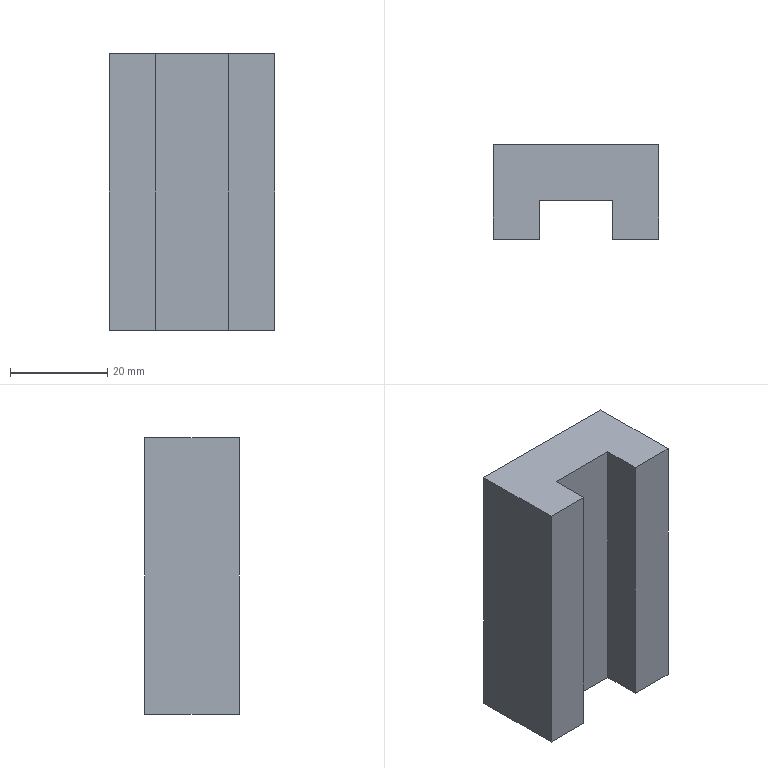Part | SolidWorks | features ICE 2, Extrusion 1 | 1 solid | 22 faces | box 34 x 19.5 x 56.8 mm | volume 30598 mm3 | plane 14 | cylinder 8 | commonest cylinder face diameters 3.6 x8
STEP:
#1=CARTESIAN_POINT('',(-13.,3.75,11.2));
#2=VERTEX_POINT('',#1);
#3=CARTESIAN_POINT('',(-13.,3.75,14.8));
#4=VERTEX_POINT('',#3);
#5=CARTESIAN_POINT('',(-13.,3.75,13.));
#6=DIRECTION('',(0.,1.,0.));
#7=DIRECTION('',(0.,0.,-1.));
#8=AXIS2_PLACEMENT_3D('',#5,#6,#7);
#9=CIRCLE('',#8,1.8);
#10=EDGE_CURVE('',#2,#4,#9,.T.);
#11=ORIENTED_EDGE('',*,*,#10,.F.);
#12=CARTESIAN_POINT('',(-13.,9.75,11.2));
#13=VERTEX_POINT('',#12);
#14=CARTESIAN_POINT('',(-13.,3.75,11.2));
#15=DIRECTION('',(0.,1.,0.));
#16=VECTOR('',#15,1000.);
#17=LINE('',#14,#16);
#18=EDGE_CURVE('',#2,#13,#17,.T.);
#19=ORIENTED_EDGE('',*,*,#18,.T.);
#20=CARTESIAN_POINT('',(-13.,9.75,14.8));
#21=VERTEX_POINT('',#20);
#22=CARTESIAN_POINT('',(-13.,9.75,13.));
#23=DIRECTION('',(0.,1.,0.));
#24=DIRECTION('',(0.,0.,-1.));
#25=AXIS2_PLACEMENT_3D('',#22,#23,#24);
#26=CIRCLE('',#25,1.8);
#27=EDGE_CURVE('',#13,#21,#26,.T.);
#28=ORIENTED_EDGE('',*,*,#27,.T.);
#29=CARTESIAN_POINT('',(-13.,3.75,14.8));
#30=DIRECTION('',(0.,1.,0.));
#31=VECTOR('',#30,1000.);
#32=LINE('',#29,#31);
#33=EDGE_CURVE('',#4,#21,#32,.T.);
#34=ORIENTED_EDGE('',*,*,#33,.F.);
#35=EDGE_LOOP('',(#11,#19,#28,#34));
#36=FACE_OUTER_BOUND('',#35,.T.);
#37=CARTESIAN_POINT('',(-13.,3.75,13.));
#38=DIRECTION('',(0.,1.,0.));
#39=DIRECTION('',(0.,0.,1.));
#40=AXIS2_PLACEMENT_3D('',#37,#38,#39);
#41=CYLINDRICAL_SURFACE('',#40,1.8);
#42=ADVANCED_FACE('',(#36),#41,.F.);
#43=CARTESIAN_POINT('',(13.,3.75,11.2));
#44=VERTEX_POINT('',#43);
#45=CARTESIAN_POINT('',(13.,3.75,14.8));
#46=VERTEX_POINT('',#45);
#47=CARTESIAN_POINT('',(13.,3.75,13.));
#48=DIRECTION('',(0.,1.,0.));
#49=DIRECTION('',(0.,0.,1.));
#50=AXIS2_PLACEMENT_3D('',#47,#48,#49);
#51=CIRCLE('',#50,1.8);
#52=EDGE_CURVE('',#44,#46,#51,.T.);
#53=ORIENTED_EDGE('',*,*,#52,.F.);
#54=CARTESIAN_POINT('',(13.,9.75,11.2));
#55=VERTEX_POINT('',#54);
#56=CARTESIAN_POINT('',(13.,3.75,11.2));
#57=DIRECTION('',(0.,1.,0.));
#58=VECTOR('',#57,1000.);
#59=LINE('',#56,#58);
#60=EDGE_CURVE('',#44,#55,#59,.T.);
#61=ORIENTED_EDGE('',*,*,#60,.T.);
#62=CARTESIAN_POINT('',(13.,9.75,14.8));
#63=VERTEX_POINT('',#62);
#64=CARTESIAN_POINT('',(13.,9.75,13.));
#65=DIRECTION('',(0.,1.,0.));
#66=DIRECTION('',(0.,0.,1.));
#67=AXIS2_PLACEMENT_3D('',#64,#65,#66);
#68=CIRCLE('',#67,1.8);
#69=EDGE_CURVE('',#55,#63,#68,.T.);
#70=ORIENTED_EDGE('',*,*,#69,.T.);
#71=CARTESIAN_POINT('',(13.,3.75,14.8));
#72=DIRECTION('',(0.,1.,0.));
#73=VECTOR('',#72,1000.);
#74=LINE('',#71,#73);
#75=EDGE_CURVE('',#46,#63,#74,.T.);
#76=ORIENTED_EDGE('',*,*,#75,.F.);
#77=EDGE_LOOP('',(#53,#61,#70,#76));
#78=FACE_OUTER_BOUND('',#77,.T.);
#79=CARTESIAN_POINT('',(13.,3.75,13.));
#80=DIRECTION('',(0.,1.,0.));
#81=DIRECTION('',(0.,0.,1.));
#82=AXIS2_PLACEMENT_3D('',#79,#80,#81);
#83=CYLINDRICAL_SURFACE('',#82,1.8);
#84=ADVANCED_FACE('',(#78),#83,.F.);
#85=CARTESIAN_POINT('',(13.,3.75,-14.8));
#86=VERTEX_POINT('',#85);
#87=CARTESIAN_POINT('',(13.,3.75,-11.2));
#88=VERTEX_POINT('',#87);
#89=CARTESIAN_POINT('',(13.,3.75,-13.));
#90=DIRECTION('',(0.,1.,0.));
#91=DIRECTION('',(0.,0.,-1.));
#92=AXIS2_PLACEMENT_3D('',#89,#90,#91);
#93=CIRCLE('',#92,1.8);
#94=EDGE_CURVE('',#86,#88,#93,.T.);
#95=ORIENTED_EDGE('',*,*,#94,.F.);
#96=CARTESIAN_POINT('',(13.,9.75,-14.8));
#97=VERTEX_POINT('',#96);
#98=CARTESIAN_POINT('',(13.,3.75,-14.8));
#99=DIRECTION('',(0.,1.,0.));
#100=VECTOR('',#99,1000.);
#101=LINE('',#98,#100);
#102=EDGE_CURVE('',#86,#97,#101,.T.);
#103=ORIENTED_EDGE('',*,*,#102,.T.);
#104=CARTESIAN_POINT('',(13.,9.75,-11.2));
#105=VERTEX_POINT('',#104);
#106=CARTESIAN_POINT('',(13.,9.75,-13.));
#107=DIRECTION('',(0.,1.,0.));
#108=DIRECTION('',(0.,0.,-1.));
#109=AXIS2_PLACEMENT_3D('',#106,#107,#108);
#110=CIRCLE('',#109,1.8);
#111=EDGE_CURVE('',#97,#105,#110,.T.);
#112=ORIENTED_EDGE('',*,*,#111,.T.);
#113=CARTESIAN_POINT('',(13.,3.75,-11.2));
#114=DIRECTION('',(0.,1.,0.));
#115=VECTOR('',#114,1000.);
#116=LINE('',#113,#115);
#117=EDGE_CURVE('',#88,#105,#116,.T.);
#118=ORIENTED_EDGE('',*,*,#117,.F.);
#119=EDGE_LOOP('',(#95,#103,#112,#118));
#120=FACE_OUTER_BOUND('',#119,.T.);
#121=CARTESIAN_POINT('',(13.,3.75,-13.));
#122=DIRECTION('',(0.,1.,0.));
#123=DIRECTION('',(0.,0.,1.));
#124=AXIS2_PLACEMENT_3D('',#121,#122,#123);
#125=CYLINDRICAL_SURFACE('',#124,1.8);
#126=ADVANCED_FACE('',(#120),#125,.F.);
#127=CARTESIAN_POINT('',(-13.,3.75,-14.8));
#128=VERTEX_POINT('',#127);
#129=CARTESIAN_POINT('',(-13.,3.75,-11.2));
#130=VERTEX_POINT('',#129);
#131=CARTESIAN_POINT('',(-13.,3.75,-13.));
#132=DIRECTION('',(0.,1.,0.));
#133=DIRECTION('',(0.,0.,1.));
#134=AXIS2_PLACEMENT_3D('',#131,#132,#133);
#135=CIRCLE('',#134,1.8);
#136=EDGE_CURVE('',#128,#130,#135,.T.);
#137=ORIENTED_EDGE('',*,*,#136,.F.);
#138=CARTESIAN_POINT('',(-13.,9.75,-14.8));
#139=VERTEX_POINT('',#138);
#140=CARTESIAN_POINT('',(-13.,3.75,-14.8));
#141=DIRECTION('',(0.,1.,0.));
#142=VECTOR('',#141,1000.);
#143=LINE('',#140,#142);
#144=EDGE_CURVE('',#128,#139,#143,.T.);
#145=ORIENTED_EDGE('',*,*,#144,.T.);
#146=CARTESIAN_POINT('',(-13.,9.75,-11.2));
#147=VERTEX_POINT('',#146);
#148=CARTESIAN_POINT('',(-13.,9.75,-13.));
#149=DIRECTION('',(0.,1.,0.));
#150=DIRECTION('',(0.,0.,1.));
#151=AXIS2_PLACEMENT_3D('',#148,#149,#150);
#152=CIRCLE('',#151,1.8);
#153=EDGE_CURVE('',#139,#147,#152,.T.);
#154=ORIENTED_EDGE('',*,*,#153,.T.);
#155=CARTESIAN_POINT('',(-13.,3.75,-11.2));
#156=DIRECTION('',(0.,1.,0.));
#157=VECTOR('',#156,1000.);
#158=LINE('',#155,#157);
#159=EDGE_CURVE('',#130,#147,#158,.T.);
#160=ORIENTED_EDGE('',*,*,#159,.F.);
#161=EDGE_LOOP('',(#137,#145,#154,#160));
#162=FACE_OUTER_BOUND('',#161,.T.);
#163=CARTESIAN_POINT('',(-13.,3.75,-13.));
#164=DIRECTION('',(0.,1.,0.));
#165=DIRECTION('',(0.,0.,1.));
#166=AXIS2_PLACEMENT_3D('',#163,#164,#165);
#167=CYLINDRICAL_SURFACE('',#166,1.8);
#168=ADVANCED_FACE('',(#162),#167,.F.);
#169=CARTESIAN_POINT('',(7.5,-9.75,28.4));
#170=VERTEX_POINT('',#169);
#171=CARTESIAN_POINT('',(17.,-9.75,28.4));
#172=VERTEX_POINT('',#171);
#173=CARTESIAN_POINT('',(-17.,-9.75,28.4));
#174=DIRECTION('',(1.,0.,0.));
#175=VECTOR('',#174,1000.);
#176=LINE('',#173,#175);
#177=EDGE_CURVE('',#170,#172,#176,.T.);
#178=ORIENTED_EDGE('',*,*,#177,.F.);
#179=CARTESIAN_POINT('',(7.5,-9.75,-28.4));
#180=VERTEX_POINT('',#179);
#181=CARTESIAN_POINT('',(7.5,-9.75,-28.4));
#182=DIRECTION('',(0.,0.,1.));
#183=VECTOR('',#182,1000.);
#184=LINE('',#181,#183);
#185=EDGE_CURVE('',#180,#170,#184,.T.);
#186=ORIENTED_EDGE('',*,*,#185,.F.);
#187=CARTESIAN_POINT('',(17.,-9.75,-28.4));
#188=VERTEX_POINT('',#187);
#189=CARTESIAN_POINT('',(-17.,-9.75,-28.4));
#190=DIRECTION('',(1.,0.,0.));
#191=VECTOR('',#190,1000.);
#192=LINE('',#189,#191);
#193=EDGE_CURVE('',#180,#188,#192,.T.);
#194=ORIENTED_EDGE('',*,*,#193,.T.);
#195=CARTESIAN_POINT('',(17.,-9.75,28.4));
#196=DIRECTION('',(0.,0.,-1.));
#197=VECTOR('',#196,1000.);
#198=LINE('',#195,#197);
#199=EDGE_CURVE('',#172,#188,#198,.T.);
#200=ORIENTED_EDGE('',*,*,#199,.F.);
#201=EDGE_LOOP('',(#178,#186,#194,#200));
#202=FACE_OUTER_BOUND('',#201,.T.);
#203=CARTESIAN_POINT('',(-17.,-9.75,28.4));
#204=DIRECTION('',(0.,1.,0.));
#205=DIRECTION('',(0.,0.,1.));
#206=AXIS2_PLACEMENT_3D('',#203,#204,#205);
#207=PLANE('',#206);
#208=ADVANCED_FACE('',(#202),#207,.F.);
#209=CARTESIAN_POINT('',(17.,9.75,-28.4));
#210=VERTEX_POINT('',#209);
#211=CARTESIAN_POINT('',(17.,9.75,-28.4));
#212=DIRECTION('',(0.,1.,0.));
#213=VECTOR('',#212,1000.);
#214=LINE('',#211,#213);
#215=EDGE_CURVE('',#188,#210,#214,.T.);
#216=ORIENTED_EDGE('',*,*,#215,.T.);
#217=CARTESIAN_POINT('',(17.,9.75,28.4));
#218=VERTEX_POINT('',#217);
#219=CARTESIAN_POINT('',(17.,9.75,28.4));
#220=DIRECTION('',(0.,0.,-1.));
#221=VECTOR('',#220,1000.);
#222=LINE('',#219,#221);
#223=EDGE_CURVE('',#218,#210,#222,.T.);
#224=ORIENTED_EDGE('',*,*,#223,.F.);
#225=CARTESIAN_POINT('',(17.,9.75,28.4));
#226=DIRECTION('',(0.,1.,0.));
#227=VECTOR('',#226,1000.);
#228=LINE('',#225,#227);
#229=EDGE_CURVE('',#172,#218,#228,.T.);
#230=ORIENTED_EDGE('',*,*,#229,.F.);
#231=ORIENTED_EDGE('',*,*,#199,.T.);
#232=EDGE_LOOP('',(#216,#224,#230,#231));
#233=FACE_OUTER_BOUND('',#232,.T.);
#234=CARTESIAN_POINT('',(17.,9.75,28.4));
#235=DIRECTION('',(-1.,0.,0.));
#236=DIRECTION('',(0.,-1.,0.));
#237=AXIS2_PLACEMENT_3D('',#234,#235,#236);
#238=PLANE('',#237);
#239=ADVANCED_FACE('',(#233),#238,.F.);
#240=CARTESIAN_POINT('',(-13.,9.75,13.));
#241=DIRECTION('',(0.,1.,0.));
#242=DIRECTION('',(0.,0.,-1.));
#243=AXIS2_PLACEMENT_3D('',#240,#241,#242);
#244=CIRCLE('',#243,1.8);
#245=EDGE_CURVE('',#21,#13,#244,.T.);
#246=ORIENTED_EDGE('',*,*,#245,.F.);
#247=ORIENTED_EDGE('',*,*,#27,.F.);
#248=EDGE_LOOP('',(#246,#247));
#249=FACE_BOUND('',#248,.T.);
#250=CARTESIAN_POINT('',(13.,9.75,13.));
#251=DIRECTION('',(0.,1.,0.));
#252=DIRECTION('',(0.,0.,1.));
#253=AXIS2_PLACEMENT_3D('',#250,#251,#252);
#254=CIRCLE('',#253,1.8);
#255=EDGE_CURVE('',#63,#55,#254,.T.);
#256=ORIENTED_EDGE('',*,*,#255,.F.);
#257=ORIENTED_EDGE('',*,*,#69,.F.);
#258=EDGE_LOOP('',(#256,#257));
#259=FACE_BOUND('',#258,.T.);
#260=CARTESIAN_POINT('',(13.,9.75,-13.));
#261=DIRECTION('',(0.,1.,0.));
#262=DIRECTION('',(0.,0.,-1.));
#263=AXIS2_PLACEMENT_3D('',#260,#261,#262);
#264=CIRCLE('',#263,1.8);
#265=EDGE_CURVE('',#105,#97,#264,.T.);
#266=ORIENTED_EDGE('',*,*,#265,.F.);
#267=ORIENTED_EDGE('',*,*,#111,.F.);
#268=EDGE_LOOP('',(#266,#267));
#269=FACE_BOUND('',#268,.T.);
#270=CARTESIAN_POINT('',(-13.,9.75,-13.));
#271=DIRECTION('',(0.,1.,0.));
#272=DIRECTION('',(0.,0.,1.));
#273=AXIS2_PLACEMENT_3D('',#270,#271,#272);
#274=CIRCLE('',#273,1.8);
#275=EDGE_CURVE('',#147,#139,#274,.T.);
#276=ORIENTED_EDGE('',*,*,#275,.F.);
#277=ORIENTED_EDGE('',*,*,#153,.F.);
#278=EDGE_LOOP('',(#276,#277));
#279=FACE_BOUND('',#278,.T.);
#280=CARTESIAN_POINT('',(-17.,9.75,-28.4));
#281=VERTEX_POINT('',#280);
#282=CARTESIAN_POINT('',(-17.,9.75,-28.4));
#283=DIRECTION('',(-1.,0.,0.));
#284=VECTOR('',#283,1000.);
#285=LINE('',#282,#284);
#286=EDGE_CURVE('',#210,#281,#285,.T.);
#287=ORIENTED_EDGE('',*,*,#286,.T.);
#288=CARTESIAN_POINT('',(-17.,9.75,28.4));
#289=VERTEX_POINT('',#288);
#290=CARTESIAN_POINT('',(-17.,9.75,28.4));
#291=DIRECTION('',(0.,0.,-1.));
#292=VECTOR('',#291,1000.);
#293=LINE('',#290,#292);
#294=EDGE_CURVE('',#289,#281,#293,.T.);
#295=ORIENTED_EDGE('',*,*,#294,.F.);
#296=CARTESIAN_POINT('',(-17.,9.75,28.4));
#297=DIRECTION('',(-1.,0.,0.));
#298=VECTOR('',#297,1000.);
#299=LINE('',#296,#298);
#300=EDGE_CURVE('',#218,#289,#299,.T.);
#301=ORIENTED_EDGE('',*,*,#300,.F.);
#302=ORIENTED_EDGE('',*,*,#223,.T.);
#303=EDGE_LOOP('',(#287,#295,#301,#302));
#304=FACE_OUTER_BOUND('',#303,.T.);
#305=CARTESIAN_POINT('',(-17.,9.75,28.4));
#306=DIRECTION('',(0.,-1.,0.));
#307=DIRECTION('',(0.,0.,-1.));
#308=AXIS2_PLACEMENT_3D('',#305,#306,#307);
#309=PLANE('',#308);
#310=ADVANCED_FACE('',(#249,#259,#269,#279,#304),#309,.F.);
#311=CARTESIAN_POINT('',(-17.,-9.75,-28.4));
#312=VERTEX_POINT('',#311);
#313=CARTESIAN_POINT('',(-17.,9.75,-28.4));
#314=DIRECTION('',(0.,-1.,0.));
#315=VECTOR('',#314,1000.);
#316=LINE('',#313,#315);
#317=EDGE_CURVE('',#281,#312,#316,.T.);
#318=ORIENTED_EDGE('',*,*,#317,.T.);
#319=CARTESIAN_POINT('',(-17.,-9.75,28.4));
#320=VERTEX_POINT('',#319);
#321=CARTESIAN_POINT('',(-17.,-9.75,28.4));
#322=DIRECTION('',(0.,0.,-1.));
#323=VECTOR('',#322,1000.);
#324=LINE('',#321,#323);
#325=EDGE_CURVE('',#320,#312,#324,.T.);
#326=ORIENTED_EDGE('',*,*,#325,.F.);
#327=CARTESIAN_POINT('',(-17.,9.75,28.4));
#328=DIRECTION('',(0.,-1.,0.));
#329=VECTOR('',#328,1000.);
#330=LINE('',#327,#329);
#331=EDGE_CURVE('',#289,#320,#330,.T.);
#332=ORIENTED_EDGE('',*,*,#331,.F.);
#333=ORIENTED_EDGE('',*,*,#294,.T.);
#334=EDGE_LOOP('',(#318,#326,#332,#333));
#335=FACE_OUTER_BOUND('',#334,.T.);
#336=CARTESIAN_POINT('',(-17.,9.75,28.4));
#337=DIRECTION('',(1.,0.,0.));
#338=DIRECTION('',(0.,1.,0.));
#339=AXIS2_PLACEMENT_3D('',#336,#337,#338);
#340=PLANE('',#339);
#341=ADVANCED_FACE('',(#335),#340,.F.);
#342=CARTESIAN_POINT('',(-7.5,-9.75,-28.4));
#343=VERTEX_POINT('',#342);
#344=CARTESIAN_POINT('',(-17.,-9.75,-28.4));
#345=DIRECTION('',(1.,0.,0.));
#346=VECTOR('',#345,1000.);
#347=LINE('',#344,#346);
#348=EDGE_CURVE('',#312,#343,#347,.T.);
#349=ORIENTED_EDGE('',*,*,#348,.T.);
#350=CARTESIAN_POINT('',(-7.5,-9.75,28.4));
#351=VERTEX_POINT('',#350);
#352=CARTESIAN_POINT('',(-7.5,-9.75,-28.4));
#353=DIRECTION('',(0.,0.,1.));
#354=VECTOR('',#353,1000.);
#355=LINE('',#352,#354);
#356=EDGE_CURVE('',#343,#351,#355,.T.);
#357=ORIENTED_EDGE('',*,*,#356,.T.);
#358=CARTESIAN_POINT('',(-17.,-9.75,28.4));
#359=DIRECTION('',(1.,0.,0.));
#360=VECTOR('',#359,1000.);
#361=LINE('',#358,#360);
#362=EDGE_CURVE('',#320,#351,#361,.T.);
#363=ORIENTED_EDGE('',*,*,#362,.F.);
#364=ORIENTED_EDGE('',*,*,#325,.T.);
#365=EDGE_LOOP('',(#349,#357,#363,#364));
#366=FACE_OUTER_BOUND('',#365,.T.);
#367=CARTESIAN_POINT('',(-17.,-9.75,28.4));
#368=DIRECTION('',(0.,1.,0.));
#369=DIRECTION('',(0.,0.,1.));
#370=AXIS2_PLACEMENT_3D('',#367,#368,#369);
#371=PLANE('',#370);
#372=ADVANCED_FACE('',(#366),#371,.F.);
#373=CARTESIAN_POINT('',(7.5,-1.75,28.4));
#374=VERTEX_POINT('',#373);
#375=CARTESIAN_POINT('',(7.5,-1.75,28.4));
#376=DIRECTION('',(0.,1.,0.));
#377=VECTOR('',#376,1000.);
#378=LINE('',#375,#377);
#379=EDGE_CURVE('',#170,#374,#378,.T.);
#380=ORIENTED_EDGE('',*,*,#379,.F.);
#381=ORIENTED_EDGE('',*,*,#177,.T.);
#382=ORIENTED_EDGE('',*,*,#229,.T.);
#383=ORIENTED_EDGE('',*,*,#300,.T.);
#384=ORIENTED_EDGE('',*,*,#331,.T.);
#385=ORIENTED_EDGE('',*,*,#362,.T.);
#386=CARTESIAN_POINT('',(-7.5,-1.75,28.4));
#387=VERTEX_POINT('',#386);
#388=CARTESIAN_POINT('',(-7.5,-1.75,28.4));
#389=DIRECTION('',(0.,-1.,0.));
#390=VECTOR('',#389,1000.);
#391=LINE('',#388,#390);
#392=EDGE_CURVE('',#387,#351,#391,.T.);
#393=ORIENTED_EDGE('',*,*,#392,.F.);
#394=CARTESIAN_POINT('',(-7.5,-1.75,28.4));
#395=DIRECTION('',(-1.,0.,0.));
#396=VECTOR('',#395,1000.);
#397=LINE('',#394,#396);
#398=EDGE_CURVE('',#374,#387,#397,.T.);
#399=ORIENTED_EDGE('',*,*,#398,.F.);
#400=EDGE_LOOP('',(#380,#381,#382,#383,#384,#385,#393,#399));
#401=FACE_OUTER_BOUND('',#400,.T.);
#402=CARTESIAN_POINT('',(0.,0.,28.4));
#403=DIRECTION('',(0.,0.,1.));
#404=DIRECTION('',(1.,0.,0.));
#405=AXIS2_PLACEMENT_3D('',#402,#403,#404);
#406=PLANE('',#405);
#407=ADVANCED_FACE('',(#401),#406,.T.);
#408=ORIENTED_EDGE('',*,*,#193,.F.);
#409=CARTESIAN_POINT('',(7.5,-1.75,-28.4));
#410=VERTEX_POINT('',#409);
#411=CARTESIAN_POINT('',(7.5,-1.75,-28.4));
#412=DIRECTION('',(0.,1.,0.));
#413=VECTOR('',#412,1000.);
#414=LINE('',#411,#413);
#415=EDGE_CURVE('',#180,#410,#414,.T.);
#416=ORIENTED_EDGE('',*,*,#415,.T.);
#417=CARTESIAN_POINT('',(-7.5,-1.75,-28.4));
#418=VERTEX_POINT('',#417);
#419=CARTESIAN_POINT('',(-7.5,-1.75,-28.4));
#420=DIRECTION('',(-1.,0.,0.));
#421=VECTOR('',#420,1000.);
#422=LINE('',#419,#421);
#423=EDGE_CURVE('',#410,#418,#422,.T.);
#424=ORIENTED_EDGE('',*,*,#423,.T.);
#425=CARTESIAN_POINT('',(-7.5,-1.75,-28.4));
#426=DIRECTION('',(0.,-1.,0.));
#427=VECTOR('',#426,1000.);
#428=LINE('',#425,#427);
#429=EDGE_CURVE('',#418,#343,#428,.T.);
#430=ORIENTED_EDGE('',*,*,#429,.T.);
#431=ORIENTED_EDGE('',*,*,#348,.F.);
#432=ORIENTED_EDGE('',*,*,#317,.F.);
#433=ORIENTED_EDGE('',*,*,#286,.F.);
#434=ORIENTED_EDGE('',*,*,#215,.F.);
#435=EDGE_LOOP('',(#408,#416,#424,#430,#431,#432,#433,#434));
#436=FACE_OUTER_BOUND('',#435,.T.);
#437=CARTESIAN_POINT('',(0.,0.,-28.4));
#438=DIRECTION('',(0.,0.,1.));
#439=DIRECTION('',(1.,0.,0.));
#440=AXIS2_PLACEMENT_3D('',#437,#438,#439);
#441=PLANE('',#440);
#442=ADVANCED_FACE('',(#436),#441,.F.);
#443=CARTESIAN_POINT('',(7.5,-1.75,-28.4));
#444=DIRECTION('',(0.,0.,1.));
#445=VECTOR('',#444,1000.);
#446=LINE('',#443,#445);
#447=EDGE_CURVE('',#410,#374,#446,.T.);
#448=ORIENTED_EDGE('',*,*,#447,.F.);
#449=ORIENTED_EDGE('',*,*,#415,.F.);
#450=ORIENTED_EDGE('',*,*,#185,.T.);
#451=ORIENTED_EDGE('',*,*,#379,.T.);
#452=EDGE_LOOP('',(#448,#449,#450,#451));
#453=FACE_OUTER_BOUND('',#452,.T.);
#454=CARTESIAN_POINT('',(7.5,-1.75,-28.4));
#455=DIRECTION('',(1.,0.,0.));
#456=DIRECTION('',(0.,1.,0.));
#457=AXIS2_PLACEMENT_3D('',#454,#455,#456);
#458=PLANE('',#457);
#459=ADVANCED_FACE('',(#453),#458,.F.);
#460=ORIENTED_EDGE('',*,*,#356,.F.);
#461=ORIENTED_EDGE('',*,*,#429,.F.);
#462=CARTESIAN_POINT('',(-7.5,-1.75,-28.4));
#463=DIRECTION('',(0.,0.,1.));
#464=VECTOR('',#463,1000.);
#465=LINE('',#462,#464);
#466=EDGE_CURVE('',#418,#387,#465,.T.);
#467=ORIENTED_EDGE('',*,*,#466,.T.);
#468=ORIENTED_EDGE('',*,*,#392,.T.);
#469=EDGE_LOOP('',(#460,#461,#467,#468));
#470=FACE_OUTER_BOUND('',#469,.T.);
#471=CARTESIAN_POINT('',(-7.5,-1.75,-28.4));
#472=DIRECTION('',(-1.,0.,0.));
#473=DIRECTION('',(0.,-1.,0.));
#474=AXIS2_PLACEMENT_3D('',#471,#472,#473);
#475=PLANE('',#474);
#476=ADVANCED_FACE('',(#470),#475,.F.);
#477=ORIENTED_EDGE('',*,*,#466,.F.);
#478=ORIENTED_EDGE('',*,*,#423,.F.);
#479=ORIENTED_EDGE('',*,*,#447,.T.);
#480=ORIENTED_EDGE('',*,*,#398,.T.);
#481=EDGE_LOOP('',(#477,#478,#479,#480));
#482=FACE_OUTER_BOUND('',#481,.T.);
#483=CARTESIAN_POINT('',(-7.5,-1.75,-28.4));
#484=DIRECTION('',(0.,1.,0.));
#485=DIRECTION('',(0.,0.,1.));
#486=AXIS2_PLACEMENT_3D('',#483,#484,#485);
#487=PLANE('',#486);
#488=ADVANCED_FACE('',(#482),#487,.F.);
#489=ORIENTED_EDGE('',*,*,#144,.F.);
#490=CARTESIAN_POINT('',(-13.,3.75,-13.));
#491=DIRECTION('',(0.,1.,0.));
#492=DIRECTION('',(0.,0.,1.));
#493=AXIS2_PLACEMENT_3D('',#490,#491,#492);
#494=CIRCLE('',#493,1.8);
#495=EDGE_CURVE('',#130,#128,#494,.T.);
#496=ORIENTED_EDGE('',*,*,#495,.F.);
#497=ORIENTED_EDGE('',*,*,#159,.T.);
#498=ORIENTED_EDGE('',*,*,#275,.T.);
#499=EDGE_LOOP('',(#489,#496,#497,#498));
#500=FACE_OUTER_BOUND('',#499,.T.);
#501=CARTESIAN_POINT('',(-13.,3.75,-13.));
#502=DIRECTION('',(0.,1.,0.));
#503=DIRECTION('',(0.,0.,1.));
#504=AXIS2_PLACEMENT_3D('',#501,#502,#503);
#505=CYLINDRICAL_SURFACE('',#504,1.8);
#506=ADVANCED_FACE('',(#500),#505,.F.);
#507=ORIENTED_EDGE('',*,*,#495,.T.);
#508=ORIENTED_EDGE('',*,*,#136,.T.);
#509=EDGE_LOOP('',(#507,#508));
#510=FACE_OUTER_BOUND('',#509,.T.);
#511=CARTESIAN_POINT('',(-13.,3.75,-13.));
#512=DIRECTION('',(0.,1.,0.));
#513=DIRECTION('',(0.,0.,1.));
#514=AXIS2_PLACEMENT_3D('',#511,#512,#513);
#515=PLANE('',#514);
#516=ADVANCED_FACE('',(#510),#515,.T.);
#517=ORIENTED_EDGE('',*,*,#102,.F.);
#518=CARTESIAN_POINT('',(13.,3.75,-13.));
#519=DIRECTION('',(0.,1.,0.));
#520=DIRECTION('',(0.,0.,-1.));
#521=AXIS2_PLACEMENT_3D('',#518,#519,#520);
#522=CIRCLE('',#521,1.8);
#523=EDGE_CURVE('',#88,#86,#522,.T.);
#524=ORIENTED_EDGE('',*,*,#523,.F.);
#525=ORIENTED_EDGE('',*,*,#117,.T.);
#526=ORIENTED_EDGE('',*,*,#265,.T.);
#527=EDGE_LOOP('',(#517,#524,#525,#526));
#528=FACE_OUTER_BOUND('',#527,.T.);
#529=CARTESIAN_POINT('',(13.,3.75,-13.));
#530=DIRECTION('',(0.,1.,0.));
#531=DIRECTION('',(0.,0.,1.));
#532=AXIS2_PLACEMENT_3D('',#529,#530,#531);
#533=CYLINDRICAL_SURFACE('',#532,1.8);
#534=ADVANCED_FACE('',(#528),#533,.F.);
#535=ORIENTED_EDGE('',*,*,#523,.T.);
#536=ORIENTED_EDGE('',*,*,#94,.T.);
#537=EDGE_LOOP('',(#535,#536));
#538=FACE_OUTER_BOUND('',#537,.T.);
#539=CARTESIAN_POINT('',(13.,3.75,-13.));
#540=DIRECTION('',(0.,-1.,0.));
#541=DIRECTION('',(0.,0.,-1.));
#542=AXIS2_PLACEMENT_3D('',#539,#540,#541);
#543=PLANE('',#542);
#544=ADVANCED_FACE('',(#538),#543,.F.);
#545=ORIENTED_EDGE('',*,*,#60,.F.);
#546=CARTESIAN_POINT('',(13.,3.75,13.));
#547=DIRECTION('',(0.,1.,0.));
#548=DIRECTION('',(0.,0.,1.));
#549=AXIS2_PLACEMENT_3D('',#546,#547,#548);
#550=CIRCLE('',#549,1.8);
#551=EDGE_CURVE('',#46,#44,#550,.T.);
#552=ORIENTED_EDGE('',*,*,#551,.F.);
#553=ORIENTED_EDGE('',*,*,#75,.T.);
#554=ORIENTED_EDGE('',*,*,#255,.T.);
#555=EDGE_LOOP('',(#545,#552,#553,#554));
#556=FACE_OUTER_BOUND('',#555,.T.);
#557=CARTESIAN_POINT('',(13.,3.75,13.));
#558=DIRECTION('',(0.,1.,0.));
#559=DIRECTION('',(0.,0.,1.));
#560=AXIS2_PLACEMENT_3D('',#557,#558,#559);
#561=CYLINDRICAL_SURFACE('',#560,1.8);
#562=ADVANCED_FACE('',(#556),#561,.F.);
#563=ORIENTED_EDGE('',*,*,#551,.T.);
#564=ORIENTED_EDGE('',*,*,#52,.T.);
#565=EDGE_LOOP('',(#563,#564));
#566=FACE_OUTER_BOUND('',#565,.T.);
#567=CARTESIAN_POINT('',(13.,3.75,13.));
#568=DIRECTION('',(0.,1.,0.));
#569=DIRECTION('',(0.,0.,1.));
#570=AXIS2_PLACEMENT_3D('',#567,#568,#569);
#571=PLANE('',#570);
#572=ADVANCED_FACE('',(#566),#571,.T.);
#573=ORIENTED_EDGE('',*,*,#18,.F.);
#574=CARTESIAN_POINT('',(-13.,3.75,13.));
#575=DIRECTION('',(0.,1.,0.));
#576=DIRECTION('',(0.,0.,-1.));
#577=AXIS2_PLACEMENT_3D('',#574,#575,#576);
#578=CIRCLE('',#577,1.8);
#579=EDGE_CURVE('',#4,#2,#578,.T.);
#580=ORIENTED_EDGE('',*,*,#579,.F.);
#581=ORIENTED_EDGE('',*,*,#33,.T.);
#582=ORIENTED_EDGE('',*,*,#245,.T.);
#583=EDGE_LOOP('',(#573,#580,#581,#582));
#584=FACE_OUTER_BOUND('',#583,.T.);
#585=CARTESIAN_POINT('',(-13.,3.75,13.));
#586=DIRECTION('',(0.,1.,0.));
#587=DIRECTION('',(0.,0.,1.));
#588=AXIS2_PLACEMENT_3D('',#585,#586,#587);
#589=CYLINDRICAL_SURFACE('',#588,1.8);
#590=ADVANCED_FACE('',(#584),#589,.F.);
#591=ORIENTED_EDGE('',*,*,#579,.T.);
#592=ORIENTED_EDGE('',*,*,#10,.T.);
#593=EDGE_LOOP('',(#591,#592));
#594=FACE_OUTER_BOUND('',#593,.T.);
#595=CARTESIAN_POINT('',(-13.,3.75,13.));
#596=DIRECTION('',(0.,-1.,0.));
#597=DIRECTION('',(0.,0.,-1.));
#598=AXIS2_PLACEMENT_3D('',#595,#596,#597);
#599=PLANE('',#598);
#600=ADVANCED_FACE('',(#594),#599,.F.);
#601=CLOSED_SHELL('',(#42,#84,#126,#168,#208,#239,#310,#341,#372,#407,#442,#459,#476,#488,#506,#516,#534,#544,#562,#572,#590,#600));
#602=MANIFOLD_SOLID_BREP('',#601);
#603=CARTESIAN_POINT('',(0.,0.,0.));
#604=DIRECTION('',(0.,0.,1.));
#605=DIRECTION('',(1.,0.,0.));
#606=AXIS2_PLACEMENT_3D('',#603,#604,#605);
#607=(LENGTH_UNIT()NAMED_UNIT(*)SI_UNIT(.MILLI.,.METRE.));
#608=UNCERTAINTY_MEASURE_WITH_UNIT(LENGTH_MEASURE(0.00001),#607,'','');
#609=(NAMED_UNIT(*)PLANE_ANGLE_UNIT()SI_UNIT($,.RADIAN.));
#610=(NAMED_UNIT(*)SI_UNIT($,.STERADIAN.)SOLID_ANGLE_UNIT());
#611=(GEOMETRIC_REPRESENTATION_CONTEXT(3)GLOBAL_UNCERTAINTY_ASSIGNED_CONTEXT((#608))GLOBAL_UNIT_ASSIGNED_CONTEXT((#607,#609,#610))REPRESENTATION_CONTEXT('',''));
#612=ADVANCED_BREP_SHAPE_REPRESENTATION('',(#602,#606),#611);